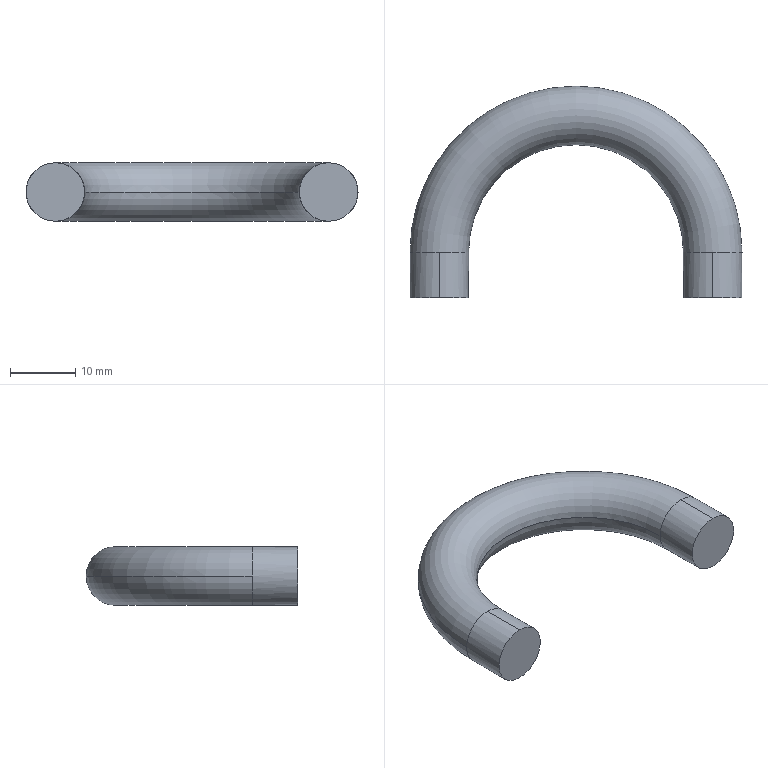Part | SolidWorks | features Sweep 1 | 1 solid | 8 faces | box 51 x 32.5 x 9 mm | volume 5088 mm3 | cylinder 4 | torus 2 | plane 2 | commonest cylinder face diameters 9 x4
STEP:
#1=CARTESIAN_POINT('',(-25.5,0.,0.));
#2=VERTEX_POINT('',#1);
#3=CARTESIAN_POINT('',(-21.,0.,-4.5));
#4=VERTEX_POINT('',#3);
#5=CARTESIAN_POINT('',(-21.,0.,0.));
#6=DIRECTION('',(0.,-1.,0.));
#7=DIRECTION('',(0.,0.,1.));
#8=AXIS2_PLACEMENT_3D('',#5,#6,#7);
#9=CIRCLE('',#8,4.5);
#10=EDGE_CURVE('',#2,#4,#9,.T.);
#11=ORIENTED_EDGE('',*,*,#10,.F.);
#12=CARTESIAN_POINT('',(25.5,0.,0.));
#13=VERTEX_POINT('',#12);
#14=CARTESIAN_POINT('',(0.,0.,0.));
#15=DIRECTION('',(0.,0.,-1.));
#16=DIRECTION('',(-1.,0.,0.));
#17=AXIS2_PLACEMENT_3D('',#14,#15,#16);
#18=CIRCLE('',#17,25.5);
#19=EDGE_CURVE('',#2,#13,#18,.T.);
#20=ORIENTED_EDGE('',*,*,#19,.T.);
#21=CARTESIAN_POINT('',(21.,0.,-4.5));
#22=VERTEX_POINT('',#21);
#23=CARTESIAN_POINT('',(21.,0.,0.));
#24=DIRECTION('',(0.,1.,0.));
#25=DIRECTION('',(0.,0.,1.));
#26=AXIS2_PLACEMENT_3D('',#23,#24,#25);
#27=CIRCLE('',#26,4.5);
#28=EDGE_CURVE('',#13,#22,#27,.T.);
#29=ORIENTED_EDGE('',*,*,#28,.T.);
#30=CARTESIAN_POINT('',(16.5,0.,0.));
#31=VERTEX_POINT('',#30);
#32=CARTESIAN_POINT('',(21.,0.,0.));
#33=DIRECTION('',(0.,1.,0.));
#34=DIRECTION('',(0.,0.,1.));
#35=AXIS2_PLACEMENT_3D('',#32,#33,#34);
#36=CIRCLE('',#35,4.5);
#37=EDGE_CURVE('',#22,#31,#36,.T.);
#38=ORIENTED_EDGE('',*,*,#37,.T.);
#39=CARTESIAN_POINT('',(-16.5,0.,0.));
#40=VERTEX_POINT('',#39);
#41=CARTESIAN_POINT('',(0.,0.,0.));
#42=DIRECTION('',(0.,0.,-1.));
#43=DIRECTION('',(-1.,0.,0.));
#44=AXIS2_PLACEMENT_3D('',#41,#42,#43);
#45=CIRCLE('',#44,16.5);
#46=EDGE_CURVE('',#40,#31,#45,.T.);
#47=ORIENTED_EDGE('',*,*,#46,.F.);
#48=CARTESIAN_POINT('',(-21.,0.,0.));
#49=DIRECTION('',(0.,-1.,0.));
#50=DIRECTION('',(0.,0.,1.));
#51=AXIS2_PLACEMENT_3D('',#48,#49,#50);
#52=CIRCLE('',#51,4.5);
#53=EDGE_CURVE('',#4,#40,#52,.T.);
#54=ORIENTED_EDGE('',*,*,#53,.F.);
#55=EDGE_LOOP('',(#11,#20,#29,#38,#47,#54));
#56=FACE_OUTER_BOUND('',#55,.T.);
#57=CARTESIAN_POINT('',(0.,0.,0.));
#58=DIRECTION('',(0.,0.,-1.));
#59=DIRECTION('',(-1.,0.,0.));
#60=AXIS2_PLACEMENT_3D('',#57,#58,#59);
#61=TOROIDAL_SURFACE('',#60,21.,4.5);
#62=ADVANCED_FACE('',(#56),#61,.T.);
#63=CARTESIAN_POINT('',(21.,0.,4.5));
#64=VERTEX_POINT('',#63);
#65=CARTESIAN_POINT('',(21.,0.,0.));
#66=DIRECTION('',(0.,1.,0.));
#67=DIRECTION('',(0.,0.,1.));
#68=AXIS2_PLACEMENT_3D('',#65,#66,#67);
#69=CIRCLE('',#68,4.5);
#70=EDGE_CURVE('',#64,#13,#69,.T.);
#71=ORIENTED_EDGE('',*,*,#70,.F.);
#72=CARTESIAN_POINT('',(21.,-7.,4.5));
#73=VERTEX_POINT('',#72);
#74=CARTESIAN_POINT('',(21.,0.,4.5));
#75=DIRECTION('',(0.,-1.,0.));
#76=VECTOR('',#75,1000.);
#77=LINE('',#74,#76);
#78=EDGE_CURVE('',#64,#73,#77,.T.);
#79=ORIENTED_EDGE('',*,*,#78,.T.);
#80=CARTESIAN_POINT('',(21.,-7.,-4.5));
#81=VERTEX_POINT('',#80);
#82=CARTESIAN_POINT('',(21.,-7.,0.));
#83=DIRECTION('',(0.,1.,0.));
#84=DIRECTION('',(0.,0.,1.));
#85=AXIS2_PLACEMENT_3D('',#82,#83,#84);
#86=CIRCLE('',#85,4.5);
#87=EDGE_CURVE('',#73,#81,#86,.T.);
#88=ORIENTED_EDGE('',*,*,#87,.T.);
#89=CARTESIAN_POINT('',(21.,0.,-4.5));
#90=DIRECTION('',(0.,-1.,0.));
#91=VECTOR('',#90,1000.);
#92=LINE('',#89,#91);
#93=EDGE_CURVE('',#22,#81,#92,.T.);
#94=ORIENTED_EDGE('',*,*,#93,.F.);
#95=ORIENTED_EDGE('',*,*,#28,.F.);
#96=EDGE_LOOP('',(#71,#79,#88,#94,#95));
#97=FACE_OUTER_BOUND('',#96,.T.);
#98=CARTESIAN_POINT('',(21.,0.,0.));
#99=DIRECTION('',(0.,-1.,0.));
#100=DIRECTION('',(0.,0.,-1.));
#101=AXIS2_PLACEMENT_3D('',#98,#99,#100);
#102=CYLINDRICAL_SURFACE('',#101,4.5);
#103=ADVANCED_FACE('',(#97),#102,.T.);
#104=CARTESIAN_POINT('',(-21.,-7.,-4.5));
#105=VERTEX_POINT('',#104);
#106=CARTESIAN_POINT('',(-21.,-7.,4.5));
#107=VERTEX_POINT('',#106);
#108=CARTESIAN_POINT('',(-21.,-7.,0.));
#109=DIRECTION('',(0.,-1.,0.));
#110=DIRECTION('',(0.,0.,1.));
#111=AXIS2_PLACEMENT_3D('',#108,#109,#110);
#112=CIRCLE('',#111,4.5);
#113=EDGE_CURVE('',#105,#107,#112,.T.);
#114=ORIENTED_EDGE('',*,*,#113,.F.);
#115=CARTESIAN_POINT('',(-21.,-7.,-4.5));
#116=DIRECTION('',(0.,1.,0.));
#117=VECTOR('',#116,1000.);
#118=LINE('',#115,#117);
#119=EDGE_CURVE('',#105,#4,#118,.T.);
#120=ORIENTED_EDGE('',*,*,#119,.T.);
#121=ORIENTED_EDGE('',*,*,#53,.T.);
#122=CARTESIAN_POINT('',(-21.,0.,4.5));
#123=VERTEX_POINT('',#122);
#124=CARTESIAN_POINT('',(-21.,0.,0.));
#125=DIRECTION('',(0.,-1.,0.));
#126=DIRECTION('',(0.,0.,1.));
#127=AXIS2_PLACEMENT_3D('',#124,#125,#126);
#128=CIRCLE('',#127,4.5);
#129=EDGE_CURVE('',#40,#123,#128,.T.);
#130=ORIENTED_EDGE('',*,*,#129,.T.);
#131=CARTESIAN_POINT('',(-21.,-7.,4.5));
#132=DIRECTION('',(0.,1.,0.));
#133=VECTOR('',#132,1000.);
#134=LINE('',#131,#133);
#135=EDGE_CURVE('',#107,#123,#134,.T.);
#136=ORIENTED_EDGE('',*,*,#135,.F.);
#137=EDGE_LOOP('',(#114,#120,#121,#130,#136));
#138=FACE_OUTER_BOUND('',#137,.T.);
#139=CARTESIAN_POINT('',(-21.,-7.,0.));
#140=DIRECTION('',(0.,1.,0.));
#141=DIRECTION('',(0.,0.,1.));
#142=AXIS2_PLACEMENT_3D('',#139,#140,#141);
#143=CYLINDRICAL_SURFACE('',#142,4.5);
#144=ADVANCED_FACE('',(#138),#143,.T.);
#145=ORIENTED_EDGE('',*,*,#78,.F.);
#146=CARTESIAN_POINT('',(21.,0.,0.));
#147=DIRECTION('',(0.,1.,0.));
#148=DIRECTION('',(0.,0.,1.));
#149=AXIS2_PLACEMENT_3D('',#146,#147,#148);
#150=CIRCLE('',#149,4.5);
#151=EDGE_CURVE('',#31,#64,#150,.T.);
#152=ORIENTED_EDGE('',*,*,#151,.F.);
#153=ORIENTED_EDGE('',*,*,#37,.F.);
#154=ORIENTED_EDGE('',*,*,#93,.T.);
#155=CARTESIAN_POINT('',(21.,-7.,0.));
#156=DIRECTION('',(0.,1.,0.));
#157=DIRECTION('',(0.,0.,1.));
#158=AXIS2_PLACEMENT_3D('',#155,#156,#157);
#159=CIRCLE('',#158,4.5);
#160=EDGE_CURVE('',#81,#73,#159,.T.);
#161=ORIENTED_EDGE('',*,*,#160,.T.);
#162=EDGE_LOOP('',(#145,#152,#153,#154,#161));
#163=FACE_OUTER_BOUND('',#162,.T.);
#164=CARTESIAN_POINT('',(21.,0.,0.));
#165=DIRECTION('',(0.,-1.,0.));
#166=DIRECTION('',(0.,0.,-1.));
#167=AXIS2_PLACEMENT_3D('',#164,#165,#166);
#168=CYLINDRICAL_SURFACE('',#167,4.5);
#169=ADVANCED_FACE('',(#163),#168,.T.);
#170=ORIENTED_EDGE('',*,*,#19,.F.);
#171=CARTESIAN_POINT('',(-21.,0.,0.));
#172=DIRECTION('',(0.,-1.,0.));
#173=DIRECTION('',(0.,0.,1.));
#174=AXIS2_PLACEMENT_3D('',#171,#172,#173);
#175=CIRCLE('',#174,4.5);
#176=EDGE_CURVE('',#123,#2,#175,.T.);
#177=ORIENTED_EDGE('',*,*,#176,.F.);
#178=ORIENTED_EDGE('',*,*,#129,.F.);
#179=ORIENTED_EDGE('',*,*,#46,.T.);
#180=ORIENTED_EDGE('',*,*,#151,.T.);
#181=ORIENTED_EDGE('',*,*,#70,.T.);
#182=EDGE_LOOP('',(#170,#177,#178,#179,#180,#181));
#183=FACE_OUTER_BOUND('',#182,.T.);
#184=CARTESIAN_POINT('',(0.,0.,0.));
#185=DIRECTION('',(0.,0.,-1.));
#186=DIRECTION('',(-1.,0.,0.));
#187=AXIS2_PLACEMENT_3D('',#184,#185,#186);
#188=TOROIDAL_SURFACE('',#187,21.,4.5);
#189=ADVANCED_FACE('',(#183),#188,.T.);
#190=ORIENTED_EDGE('',*,*,#119,.F.);
#191=CARTESIAN_POINT('',(-21.,-7.,0.));
#192=DIRECTION('',(0.,-1.,0.));
#193=DIRECTION('',(0.,0.,1.));
#194=AXIS2_PLACEMENT_3D('',#191,#192,#193);
#195=CIRCLE('',#194,4.5);
#196=EDGE_CURVE('',#107,#105,#195,.T.);
#197=ORIENTED_EDGE('',*,*,#196,.F.);
#198=ORIENTED_EDGE('',*,*,#135,.T.);
#199=ORIENTED_EDGE('',*,*,#176,.T.);
#200=ORIENTED_EDGE('',*,*,#10,.T.);
#201=EDGE_LOOP('',(#190,#197,#198,#199,#200));
#202=FACE_OUTER_BOUND('',#201,.T.);
#203=CARTESIAN_POINT('',(-21.,-7.,0.));
#204=DIRECTION('',(0.,1.,0.));
#205=DIRECTION('',(0.,0.,1.));
#206=AXIS2_PLACEMENT_3D('',#203,#204,#205);
#207=CYLINDRICAL_SURFACE('',#206,4.5);
#208=ADVANCED_FACE('',(#202),#207,.T.);
#209=ORIENTED_EDGE('',*,*,#160,.F.);
#210=ORIENTED_EDGE('',*,*,#87,.F.);
#211=EDGE_LOOP('',(#209,#210));
#212=FACE_OUTER_BOUND('',#211,.T.);
#213=CARTESIAN_POINT('',(21.,-7.,0.));
#214=DIRECTION('',(0.,1.,0.));
#215=DIRECTION('',(0.,0.,1.));
#216=AXIS2_PLACEMENT_3D('',#213,#214,#215);
#217=PLANE('',#216);
#218=ADVANCED_FACE('',(#212),#217,.F.);
#219=ORIENTED_EDGE('',*,*,#196,.T.);
#220=ORIENTED_EDGE('',*,*,#113,.T.);
#221=EDGE_LOOP('',(#219,#220));
#222=FACE_OUTER_BOUND('',#221,.T.);
#223=CARTESIAN_POINT('',(-21.,-7.,0.));
#224=DIRECTION('',(0.,-1.,0.));
#225=DIRECTION('',(0.,0.,1.));
#226=AXIS2_PLACEMENT_3D('',#223,#224,#225);
#227=PLANE('',#226);
#228=ADVANCED_FACE('',(#222),#227,.T.);
#229=CLOSED_SHELL('',(#62,#103,#144,#169,#189,#208,#218,#228));
#230=MANIFOLD_SOLID_BREP('',#229);
#231=CARTESIAN_POINT('',(0.,0.,0.));
#232=DIRECTION('',(0.,0.,1.));
#233=DIRECTION('',(1.,0.,0.));
#234=AXIS2_PLACEMENT_3D('',#231,#232,#233);
#235=(LENGTH_UNIT()NAMED_UNIT(*)SI_UNIT(.MILLI.,.METRE.));
#236=UNCERTAINTY_MEASURE_WITH_UNIT(LENGTH_MEASURE(0.00001),#235,'','');
#237=(NAMED_UNIT(*)PLANE_ANGLE_UNIT()SI_UNIT($,.RADIAN.));
#238=(NAMED_UNIT(*)SI_UNIT($,.STERADIAN.)SOLID_ANGLE_UNIT());
#239=(GEOMETRIC_REPRESENTATION_CONTEXT(3)GLOBAL_UNCERTAINTY_ASSIGNED_CONTEXT((#236))GLOBAL_UNIT_ASSIGNED_CONTEXT((#235,#237,#238))REPRESENTATION_CONTEXT('',''));
#240=ADVANCED_BREP_SHAPE_REPRESENTATION('',(#230,#234),#239);